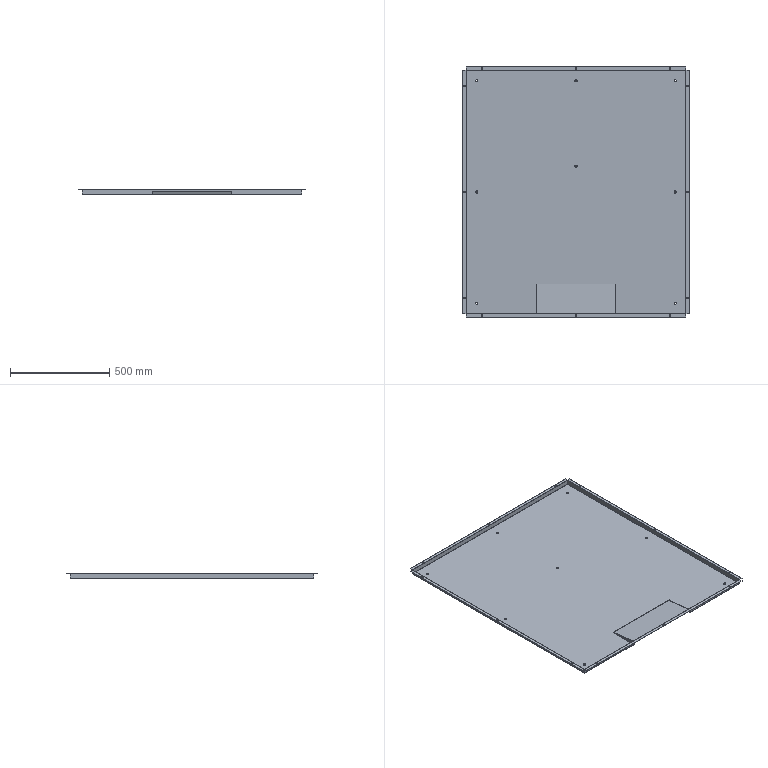Part | SolidWorks | 2 solids | 170 faces | box 1140 x 1260 x 25.087 mm | volume 1538829 mm3 | plane 90 | cylinder 68 | spline 12 | commonest cylinder face diameters 7 x30 11 x16 0.4 x9 2.4 x9 2 x2 4 x2